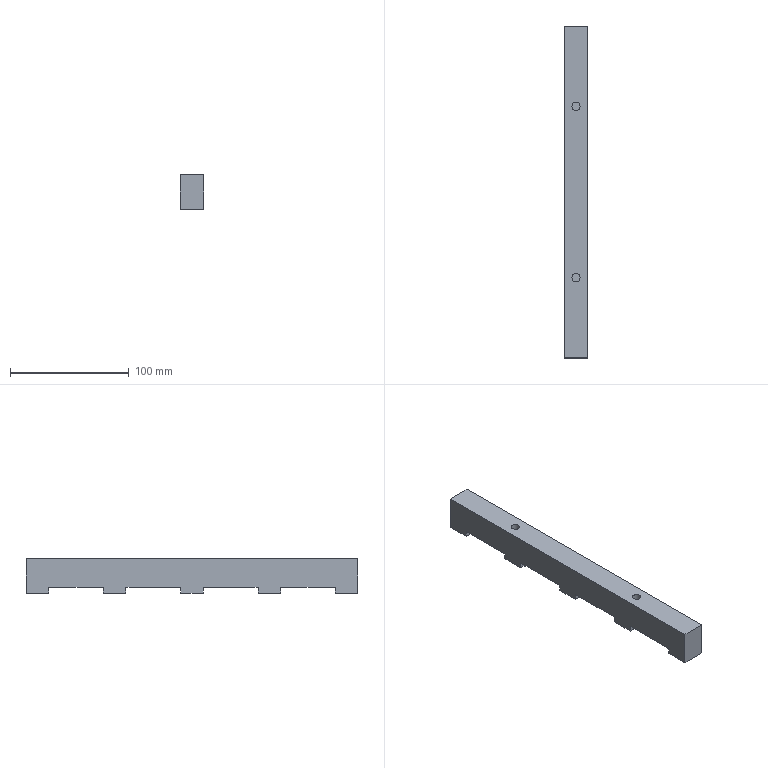CAM job | NX | 3-axis milling, drilling | part box 20 x 279 x 29 mm | stock box 25 x 284 x 35 mm
Tools:
number,name,description,diameter,corner_radius,flute_length,length,flutes
9,D10,平底铣刀-粗,10.0,0.0,35.0,75.0,2
10,D10-J,平底铣刀-精,10.0,0.0,35.0,75.0,2
1,D80R0.8飞刀,圆鼻刀-粗,80.0,0.8,50.0,75.0,2
1,D80R0.8飞刀-J,圆鼻刀-精,80.0,0.8,50.0,75.0,2
2,D6倒角刀,倒角刀,6.0,0.0,3.0,25.0,2
17,M8X1.25,丝锥,6.8,0.0,35.0,50.0,2
16,ZT6.8,钻头,6.8,0.0,35.0,50.0,2
Operations:
program,operation,operation_type,tool,method,geometry_group,spindle_rpm,surface_speed,feed_per_tooth,feed_cut,feed_plunge,cut_length_mm,path_length_mm,cut_time_min,machine_time_min
B,底壁铣飞面一刀开粗_COPY,VolumeBased25DMillingOperation,D80R0.8飞刀,分层开粗-切深K-步距G,W-B,5000.0,1256.637,0.3,3000.0,100.0,4259.134,8828.511,1.42,1.877
B,底壁铣飞面一刀精光_COPY,VolumeBased25DMillingOperation,D80R0.8飞刀-J,侧刃精光-切深K-步距G,W-B,5000.0,1256.637,0.1,1000.0,100.0,386.998,482.998,0.387,0.3966
B,底壁铣分层开粗-中_COPY,VolumeBased25DMillingOperation,D10,分层开粗-切深K-步距G,W-B,8000.0,251.32,0.25,4000.0,100.0,8977.793,9701.718,2.244,2.317
B,平面去毛刺6X45L_COPY,SurfaceContour,D6倒角刀,爬面_倒角-切深0-步距G,W-B,6500.0,122.519,0.1154,1500.0,100.0,829.551,1764.842,0.553,0.6466
B,底壁铣精光底面-中_COPY,VolumeBased25DMillingOperation,D10-J,精光步距切深关,W-B,8000.0,251.32,0.0625,1000.0,100.0,1247.833,1546.061,1.248,1.278
B,底壁铣精光侧面-中-选底面_COPY,VolumeBased25DMillingOperation,D10-J,侧刃精光-切深K-步距G,W-B,8000.0,251.32,0.0625,1000.0,100.0,306.264,596.886,0.3063,0.3353
A,顶面,FaceMilling,D80R0.8飞刀,侧刃精光-切深K-步距G,W-A,5000.0,1256.637,0.1,1000.0,100.0,373.0,409.0,0.373,0.3766
A,外形粗_2,VolumeBased25DMillingOperation,D10,METHOD,W-A,8000.0,251.327,0.3125,5000.0,80.0,24573.244,24641.244,4.915,4.921
A,打点-深0.8,Operation,D6倒角刀,NONE,W-A,8000.0,150.796,0.0312,500.0,90.0,3.6,192.203,0.0072,0.0261
A,盲锥孔-M8螺纹底孔,Operation,ZT6.8,NONE,W-A,2200.0,47.551,0.0682,300.0,90.0,34.0,253.004,0.1133,0.1352
A,仅选体,SurfaceContour,D6倒角刀,METHOD,W-A,8000.0,150.796,0.1875,3000.0,100.0,615.313,651.114,0.2051,0.2087
A,铣倒角_1,PlanarMilling,D6倒角刀,METHOD,W-A,8000.0,150.796,0.0375,600.0,100.0,49.209,279.809,0.082,0.1051
A,盲锥孔-攻牙M8,Operation,M8X1.25,METHOD,W-A,500.0,10.681,0.0013,1.25,90.0,26.0,237.004,20.8,20.821
A,外形半精_2,VolumeBased25DMillingOperation,D10-J,METHOD,W-A,8000.0,251.327,0.0625,1000.0,100.0,1268.748,1437.763,1.269,1.286